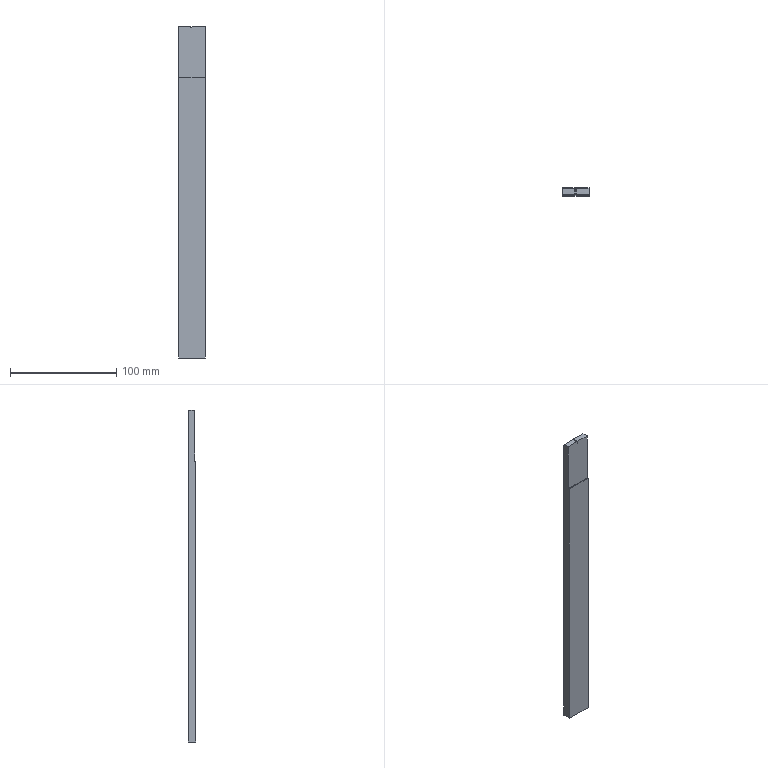Part | STEP file | P011002L003-000 | 1 solid | 86 faces | box 25 x 7.502 x 312.004 mm | volume 56592 mm3 | plane 49 | spline 11 | cone 10 | other 10 | cylinder 6 | commonest cylinder face diameters 4.167 x2 4.983 x2 5 x2